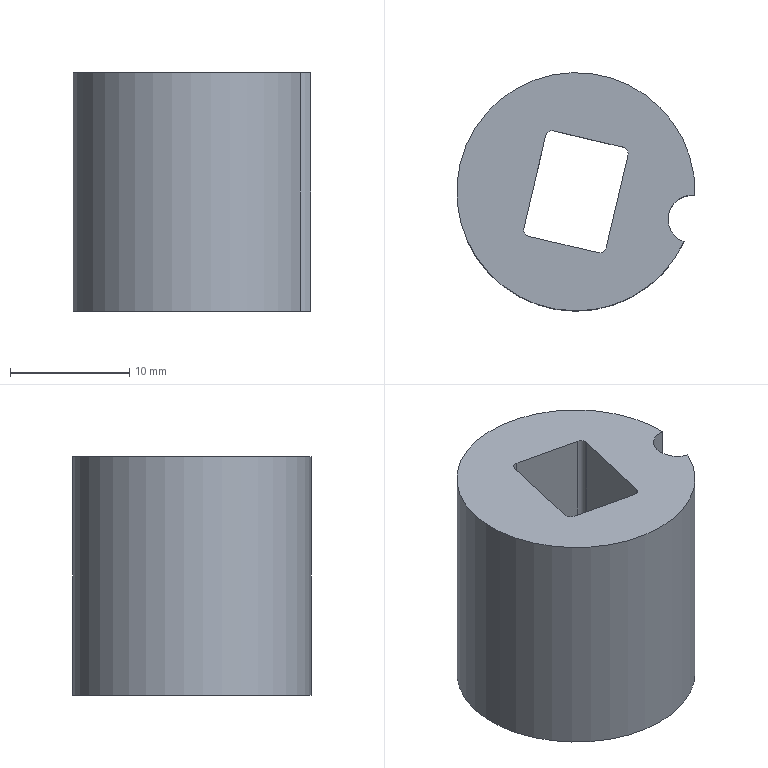Part | NX | features solid 2 | 1 solid | 14 faces | box 20 x 20 x 20 mm | volume 4152 mm3 | cylinder 7 | plane 7 | commonest cylinder face diameters 1.1 x4 4 x1 12.6 x1 20 x1
STEP:
#1=CARTESIAN_POINT('',(-482.896,-233.019,31.));
#2=VERTEX_POINT('',#1);
#3=CARTESIAN_POINT('',(-482.896,-233.019,51.));
#4=VERTEX_POINT('',#3);
#5=CARTESIAN_POINT('',(-482.896,-233.019,41.));
#6=DIRECTION('',(0.,0.,1.));
#7=VECTOR('',#6,1000.);
#8=LINE('',#5,#7);
#9=EDGE_CURVE('',#2,#4,#8,.T.);
#10=ORIENTED_EDGE('',*,*,#9,.F.);
#11=CARTESIAN_POINT('',(-483.808,-236.893,31.));
#12=VERTEX_POINT('',#11);
#13=CARTESIAN_POINT('',(-492.891,-232.711,31.));
#14=DIRECTION('',(0.,0.,1.));
#15=DIRECTION('',(0.9734,-0.2291,0.));
#16=AXIS2_PLACEMENT_3D('',#13,#14,#15);
#17=CIRCLE('',#16,10.);
#18=EDGE_CURVE('',#2,#12,#17,.T.);
#19=ORIENTED_EDGE('',*,*,#18,.T.);
#20=CARTESIAN_POINT('',(-483.808,-236.893,51.));
#21=VERTEX_POINT('',#20);
#22=CARTESIAN_POINT('',(-483.808,-236.893,41.));
#23=DIRECTION('',(0.,0.,1.));
#24=VECTOR('',#23,1000.);
#25=LINE('',#22,#24);
#26=EDGE_CURVE('',#21,#12,#25,.F.);
#27=ORIENTED_EDGE('',*,*,#26,.F.);
#28=CARTESIAN_POINT('',(-492.891,-232.711,51.));
#29=DIRECTION('',(0.,0.,1.));
#30=DIRECTION('',(0.9734,-0.2291,0.));
#31=AXIS2_PLACEMENT_3D('',#28,#29,#30);
#32=CIRCLE('',#31,10.);
#33=EDGE_CURVE('',#4,#21,#32,.T.);
#34=ORIENTED_EDGE('',*,*,#33,.F.);
#35=EDGE_LOOP('',(#10,#19,#27,#34));
#36=FACE_BOUND('',#35,.T.);
#37=CARTESIAN_POINT('',(-492.891,-232.711,31.));
#38=DIRECTION('',(0.,0.,1.));
#39=DIRECTION('',(0.9734,-0.2291,0.));
#40=AXIS2_PLACEMENT_3D('',#37,#38,#39);
#41=CYLINDRICAL_SURFACE('',#40,10.);
#42=ADVANCED_FACE('',(#36),#41,.T.);
#43=CARTESIAN_POINT('',(-486.759,-234.155,31.));
#44=VERTEX_POINT('',#43);
#45=CARTESIAN_POINT('',(-492.891,-232.711,31.));
#46=DIRECTION('',(0.,0.,1.));
#47=DIRECTION('',(0.9734,-0.2291,0.));
#48=AXIS2_PLACEMENT_3D('',#45,#46,#47);
#49=CIRCLE('',#48,6.3);
#50=EDGE_CURVE('',#44,#44,#49,.T.);
#51=ORIENTED_EDGE('',*,*,#50,.T.);
#52=EDGE_LOOP('',(#51));
#53=FACE_BOUND('',#52,.T.);
#54=ORIENTED_EDGE('',*,*,#18,.F.);
#55=CARTESIAN_POINT('',(-483.157,-235.002,31.));
#56=DIRECTION('',(0.,0.,1.));
#57=DIRECTION('',(0.9734,-0.2291,0.));
#58=AXIS2_PLACEMENT_3D('',#55,#56,#57);
#59=CIRCLE('',#58,2.);
#60=EDGE_CURVE('',#2,#12,#59,.T.);
#61=ORIENTED_EDGE('',*,*,#60,.T.);
#62=EDGE_LOOP('',(#54,#61));
#63=FACE_BOUND('',#62,.T.);
#64=CARTESIAN_POINT('',(-492.891,-232.711,31.));
#65=DIRECTION('',(0.,0.,1.));
#66=DIRECTION('',(0.9734,-0.2291,0.));
#67=AXIS2_PLACEMENT_3D('',#64,#65,#66);
#68=PLANE('',#67);
#69=ADVANCED_FACE('',(#53,#63),#68,.F.);
#70=CARTESIAN_POINT('',(-495.43,-228.004,51.));
#71=VERTEX_POINT('',#70);
#72=CARTESIAN_POINT('',(-497.263,-235.791,51.));
#73=VERTEX_POINT('',#72);
#74=CARTESIAN_POINT('',(-495.304,-227.469,51.));
#75=DIRECTION('',(-0.2291,-0.9734,0.));
#76=VECTOR('',#75,1000.);
#77=LINE('',#74,#76);
#78=EDGE_CURVE('',#71,#73,#77,.T.);
#79=ORIENTED_EDGE('',*,*,#78,.F.);
#80=CARTESIAN_POINT('',(-494.769,-227.595,51.));
#81=VERTEX_POINT('',#80);
#82=CARTESIAN_POINT('',(-494.895,-228.13,51.));
#83=DIRECTION('',(0.,0.,1.));
#84=DIRECTION('',(0.9734,-0.2291,0.));
#85=AXIS2_PLACEMENT_3D('',#82,#83,#84);
#86=CIRCLE('',#85,0.55);
#87=EDGE_CURVE('',#71,#81,#86,.F.);
#88=ORIENTED_EDGE('',*,*,#87,.T.);
#89=CARTESIAN_POINT('',(-488.929,-228.97,51.));
#90=VERTEX_POINT('',#89);
#91=CARTESIAN_POINT('',(-488.393,-229.096,51.));
#92=DIRECTION('',(-0.9734,0.2291,0.));
#93=VECTOR('',#92,1000.);
#94=LINE('',#91,#93);
#95=EDGE_CURVE('',#90,#81,#94,.T.);
#96=ORIENTED_EDGE('',*,*,#95,.F.);
#97=CARTESIAN_POINT('',(-488.519,-229.631,51.));
#98=VERTEX_POINT('',#97);
#99=CARTESIAN_POINT('',(-489.055,-229.505,51.));
#100=DIRECTION('',(0.,0.,1.));
#101=DIRECTION('',(0.9734,-0.2291,0.));
#102=AXIS2_PLACEMENT_3D('',#99,#100,#101);
#103=CIRCLE('',#102,0.55);
#104=EDGE_CURVE('',#90,#98,#103,.F.);
#105=ORIENTED_EDGE('',*,*,#104,.T.);
#106=CARTESIAN_POINT('',(-490.352,-237.418,51.));
#107=VERTEX_POINT('',#106);
#108=CARTESIAN_POINT('',(-488.393,-229.096,51.));
#109=DIRECTION('',(-0.2291,-0.9734,0.));
#110=VECTOR('',#109,1000.);
#111=LINE('',#108,#110);
#112=EDGE_CURVE('',#98,#107,#111,.T.);
#113=ORIENTED_EDGE('',*,*,#112,.T.);
#114=CARTESIAN_POINT('',(-491.014,-237.827,51.));
#115=VERTEX_POINT('',#114);
#116=CARTESIAN_POINT('',(-490.888,-237.292,51.));
#117=DIRECTION('',(0.,0.,1.));
#118=DIRECTION('',(0.9734,-0.2291,0.));
#119=AXIS2_PLACEMENT_3D('',#116,#117,#118);
#120=CIRCLE('',#119,0.55);
#121=EDGE_CURVE('',#107,#115,#120,.F.);
#122=ORIENTED_EDGE('',*,*,#121,.T.);
#123=CARTESIAN_POINT('',(-496.854,-236.453,51.));
#124=VERTEX_POINT('',#123);
#125=CARTESIAN_POINT('',(-497.389,-236.327,51.));
#126=DIRECTION('',(0.9734,-0.2291,0.));
#127=VECTOR('',#126,1000.);
#128=LINE('',#125,#127);
#129=EDGE_CURVE('',#124,#115,#128,.T.);
#130=ORIENTED_EDGE('',*,*,#129,.F.);
#131=CARTESIAN_POINT('',(-496.728,-235.917,51.));
#132=DIRECTION('',(0.,0.,1.));
#133=DIRECTION('',(0.9734,-0.2291,0.));
#134=AXIS2_PLACEMENT_3D('',#131,#132,#133);
#135=CIRCLE('',#134,0.55);
#136=EDGE_CURVE('',#124,#73,#135,.F.);
#137=ORIENTED_EDGE('',*,*,#136,.T.);
#138=EDGE_LOOP('',(#79,#88,#96,#105,#113,#122,#130,#137));
#139=FACE_BOUND('',#138,.T.);
#140=CARTESIAN_POINT('',(-483.157,-235.002,51.));
#141=DIRECTION('',(0.,0.,1.));
#142=DIRECTION('',(0.9734,-0.2291,0.));
#143=AXIS2_PLACEMENT_3D('',#140,#141,#142);
#144=CIRCLE('',#143,2.);
#145=EDGE_CURVE('',#4,#21,#144,.T.);
#146=ORIENTED_EDGE('',*,*,#145,.F.);
#147=ORIENTED_EDGE('',*,*,#33,.T.);
#148=EDGE_LOOP('',(#146,#147));
#149=FACE_BOUND('',#148,.T.);
#150=CARTESIAN_POINT('',(-492.891,-232.711,51.));
#151=DIRECTION('',(0.,0.,1.));
#152=DIRECTION('',(0.9734,-0.2291,0.));
#153=AXIS2_PLACEMENT_3D('',#150,#151,#152);
#154=PLANE('',#153);
#155=ADVANCED_FACE('',(#139,#149),#154,.T.);
#156=ORIENTED_EDGE('',*,*,#50,.F.);
#157=EDGE_LOOP('',(#156));
#158=FACE_BOUND('',#157,.T.);
#159=CARTESIAN_POINT('',(-486.759,-234.155,43.));
#160=VERTEX_POINT('',#159);
#161=CARTESIAN_POINT('',(-492.891,-232.711,43.));
#162=DIRECTION('',(0.,0.,1.));
#163=DIRECTION('',(0.9734,-0.2291,0.));
#164=AXIS2_PLACEMENT_3D('',#161,#162,#163);
#165=CIRCLE('',#164,6.3);
#166=EDGE_CURVE('',#160,#160,#165,.T.);
#167=ORIENTED_EDGE('',*,*,#166,.T.);
#168=EDGE_LOOP('',(#167));
#169=FACE_BOUND('',#168,.T.);
#170=CARTESIAN_POINT('',(-492.891,-232.711,31.));
#171=DIRECTION('',(0.,0.,1.));
#172=DIRECTION('',(0.9734,-0.2291,0.));
#173=AXIS2_PLACEMENT_3D('',#170,#171,#172);
#174=CYLINDRICAL_SURFACE('',#173,6.3);
#175=ADVANCED_FACE('',(#158,#169),#174,.F.);
#176=CARTESIAN_POINT('',(-488.519,-229.631,43.));
#177=VERTEX_POINT('',#176);
#178=CARTESIAN_POINT('',(-490.352,-237.418,43.));
#179=VERTEX_POINT('',#178);
#180=CARTESIAN_POINT('',(-489.436,-233.524,43.));
#181=DIRECTION('',(-0.2291,-0.9734,0.));
#182=VECTOR('',#181,1000.);
#183=LINE('',#180,#182);
#184=EDGE_CURVE('',#177,#179,#183,.T.);
#185=ORIENTED_EDGE('',*,*,#184,.F.);
#186=CARTESIAN_POINT('',(-488.929,-228.97,43.));
#187=VERTEX_POINT('',#186);
#188=CARTESIAN_POINT('',(-489.055,-229.505,43.));
#189=DIRECTION('',(0.,0.,1.));
#190=DIRECTION('',(0.9734,-0.2291,0.));
#191=AXIS2_PLACEMENT_3D('',#188,#189,#190);
#192=CIRCLE('',#191,0.55);
#193=EDGE_CURVE('',#177,#187,#192,.T.);
#194=ORIENTED_EDGE('',*,*,#193,.T.);
#195=CARTESIAN_POINT('',(-494.769,-227.595,43.));
#196=VERTEX_POINT('',#195);
#197=CARTESIAN_POINT('',(-491.849,-228.282,43.));
#198=DIRECTION('',(-0.9734,0.2291,0.));
#199=VECTOR('',#198,1000.);
#200=LINE('',#197,#199);
#201=EDGE_CURVE('',#187,#196,#200,.T.);
#202=ORIENTED_EDGE('',*,*,#201,.T.);
#203=CARTESIAN_POINT('',(-495.43,-228.004,43.));
#204=VERTEX_POINT('',#203);
#205=CARTESIAN_POINT('',(-494.895,-228.13,43.));
#206=DIRECTION('',(0.,0.,1.));
#207=DIRECTION('',(0.9734,-0.2291,0.));
#208=AXIS2_PLACEMENT_3D('',#205,#206,#207);
#209=CIRCLE('',#208,0.55);
#210=EDGE_CURVE('',#196,#204,#209,.T.);
#211=ORIENTED_EDGE('',*,*,#210,.T.);
#212=CARTESIAN_POINT('',(-497.263,-235.791,43.));
#213=VERTEX_POINT('',#212);
#214=CARTESIAN_POINT('',(-496.347,-231.898,43.));
#215=DIRECTION('',(-0.2291,-0.9734,0.));
#216=VECTOR('',#215,1000.);
#217=LINE('',#214,#216);
#218=EDGE_CURVE('',#204,#213,#217,.T.);
#219=ORIENTED_EDGE('',*,*,#218,.T.);
#220=CARTESIAN_POINT('',(-496.854,-236.453,43.));
#221=VERTEX_POINT('',#220);
#222=CARTESIAN_POINT('',(-496.728,-235.917,43.));
#223=DIRECTION('',(0.,0.,1.));
#224=DIRECTION('',(0.9734,-0.2291,0.));
#225=AXIS2_PLACEMENT_3D('',#222,#223,#224);
#226=CIRCLE('',#225,0.55);
#227=EDGE_CURVE('',#213,#221,#226,.T.);
#228=ORIENTED_EDGE('',*,*,#227,.T.);
#229=CARTESIAN_POINT('',(-491.014,-237.827,43.));
#230=VERTEX_POINT('',#229);
#231=CARTESIAN_POINT('',(-493.934,-237.14,43.));
#232=DIRECTION('',(0.9734,-0.2291,0.));
#233=VECTOR('',#232,1000.);
#234=LINE('',#231,#233);
#235=EDGE_CURVE('',#221,#230,#234,.T.);
#236=ORIENTED_EDGE('',*,*,#235,.T.);
#237=CARTESIAN_POINT('',(-490.888,-237.292,43.));
#238=DIRECTION('',(0.,0.,1.));
#239=DIRECTION('',(0.9734,-0.2291,0.));
#240=AXIS2_PLACEMENT_3D('',#237,#238,#239);
#241=CIRCLE('',#240,0.55);
#242=EDGE_CURVE('',#230,#179,#241,.T.);
#243=ORIENTED_EDGE('',*,*,#242,.T.);
#244=EDGE_LOOP('',(#185,#194,#202,#211,#219,#228,#236,#243));
#245=FACE_BOUND('',#244,.T.);
#246=ORIENTED_EDGE('',*,*,#166,.F.);
#247=EDGE_LOOP('',(#246));
#248=FACE_BOUND('',#247,.T.);
#249=CARTESIAN_POINT('',(-492.891,-232.711,43.));
#250=DIRECTION('',(0.,0.,1.));
#251=DIRECTION('',(0.9734,-0.2291,0.));
#252=AXIS2_PLACEMENT_3D('',#249,#250,#251);
#253=PLANE('',#252);
#254=ADVANCED_FACE('',(#245,#248),#253,.F.);
#255=ORIENTED_EDGE('',*,*,#9,.T.);
#256=ORIENTED_EDGE('',*,*,#145,.T.);
#257=ORIENTED_EDGE('',*,*,#26,.T.);
#258=ORIENTED_EDGE('',*,*,#60,.F.);
#259=EDGE_LOOP('',(#255,#256,#257,#258));
#260=FACE_BOUND('',#259,.T.);
#261=CARTESIAN_POINT('',(-483.157,-235.002,31.));
#262=DIRECTION('',(0.,0.,1.));
#263=DIRECTION('',(0.9734,-0.2291,0.));
#264=AXIS2_PLACEMENT_3D('',#261,#262,#263);
#265=CYLINDRICAL_SURFACE('',#264,2.);
#266=ADVANCED_FACE('',(#260),#265,.F.);
#267=ORIENTED_EDGE('',*,*,#78,.T.);
#268=CARTESIAN_POINT('',(-497.263,-235.791,43.));
#269=DIRECTION('',(0.,0.,1.));
#270=VECTOR('',#269,1000.);
#271=LINE('',#268,#270);
#272=EDGE_CURVE('',#73,#213,#271,.F.);
#273=ORIENTED_EDGE('',*,*,#272,.T.);
#274=ORIENTED_EDGE('',*,*,#218,.F.);
#275=CARTESIAN_POINT('',(-495.43,-228.004,51.));
#276=DIRECTION('',(0.,0.,1.));
#277=VECTOR('',#276,1000.);
#278=LINE('',#275,#277);
#279=EDGE_CURVE('',#204,#71,#278,.T.);
#280=ORIENTED_EDGE('',*,*,#279,.T.);
#281=EDGE_LOOP('',(#267,#273,#274,#280));
#282=FACE_BOUND('',#281,.T.);
#283=CARTESIAN_POINT('',(-495.304,-227.469,31.));
#284=DIRECTION('',(-0.9734,0.2291,0.));
#285=DIRECTION('',(0.,0.,1.));
#286=AXIS2_PLACEMENT_3D('',#283,#284,#285);
#287=PLANE('',#286);
#288=ADVANCED_FACE('',(#282),#287,.F.);
#289=ORIENTED_EDGE('',*,*,#129,.T.);
#290=CARTESIAN_POINT('',(-491.014,-237.827,31.));
#291=DIRECTION('',(0.,0.,1.));
#292=VECTOR('',#291,1000.);
#293=LINE('',#290,#292);
#294=EDGE_CURVE('',#115,#230,#293,.F.);
#295=ORIENTED_EDGE('',*,*,#294,.T.);
#296=ORIENTED_EDGE('',*,*,#235,.F.);
#297=CARTESIAN_POINT('',(-496.854,-236.453,51.));
#298=DIRECTION('',(0.,0.,1.));
#299=VECTOR('',#298,1000.);
#300=LINE('',#297,#299);
#301=EDGE_CURVE('',#221,#124,#300,.T.);
#302=ORIENTED_EDGE('',*,*,#301,.T.);
#303=EDGE_LOOP('',(#289,#295,#296,#302));
#304=FACE_BOUND('',#303,.T.);
#305=CARTESIAN_POINT('',(-497.389,-236.327,31.));
#306=DIRECTION('',(-0.2291,-0.9734,0.));
#307=DIRECTION('',(0.,0.,-1.));
#308=AXIS2_PLACEMENT_3D('',#305,#306,#307);
#309=PLANE('',#308);
#310=ADVANCED_FACE('',(#304),#309,.F.);
#311=ORIENTED_EDGE('',*,*,#112,.F.);
#312=CARTESIAN_POINT('',(-488.519,-229.631,31.));
#313=DIRECTION('',(0.,0.,1.));
#314=VECTOR('',#313,1000.);
#315=LINE('',#312,#314);
#316=EDGE_CURVE('',#98,#177,#315,.F.);
#317=ORIENTED_EDGE('',*,*,#316,.T.);
#318=ORIENTED_EDGE('',*,*,#184,.T.);
#319=CARTESIAN_POINT('',(-490.352,-237.418,31.));
#320=DIRECTION('',(0.,0.,1.));
#321=VECTOR('',#320,1000.);
#322=LINE('',#319,#321);
#323=EDGE_CURVE('',#179,#107,#322,.T.);
#324=ORIENTED_EDGE('',*,*,#323,.T.);
#325=EDGE_LOOP('',(#311,#317,#318,#324));
#326=FACE_BOUND('',#325,.T.);
#327=CARTESIAN_POINT('',(-488.393,-229.096,31.));
#328=DIRECTION('',(-0.9734,0.2291,0.));
#329=DIRECTION('',(0.,0.,1.));
#330=AXIS2_PLACEMENT_3D('',#327,#328,#329);
#331=PLANE('',#330);
#332=ADVANCED_FACE('',(#326),#331,.T.);
#333=ORIENTED_EDGE('',*,*,#201,.F.);
#334=CARTESIAN_POINT('',(-488.929,-228.97,31.));
#335=DIRECTION('',(0.,0.,1.));
#336=VECTOR('',#335,1000.);
#337=LINE('',#334,#336);
#338=EDGE_CURVE('',#187,#90,#337,.T.);
#339=ORIENTED_EDGE('',*,*,#338,.T.);
#340=ORIENTED_EDGE('',*,*,#95,.T.);
#341=CARTESIAN_POINT('',(-494.769,-227.595,43.));
#342=DIRECTION('',(0.,0.,1.));
#343=VECTOR('',#342,1000.);
#344=LINE('',#341,#343);
#345=EDGE_CURVE('',#81,#196,#344,.F.);
#346=ORIENTED_EDGE('',*,*,#345,.T.);
#347=EDGE_LOOP('',(#333,#339,#340,#346));
#348=FACE_BOUND('',#347,.T.);
#349=CARTESIAN_POINT('',(-488.393,-229.096,31.));
#350=DIRECTION('',(0.2291,0.9734,0.));
#351=DIRECTION('',(0.,0.,1.));
#352=AXIS2_PLACEMENT_3D('',#349,#350,#351);
#353=PLANE('',#352);
#354=ADVANCED_FACE('',(#348),#353,.F.);
#355=ORIENTED_EDGE('',*,*,#193,.F.);
#356=ORIENTED_EDGE('',*,*,#316,.F.);
#357=ORIENTED_EDGE('',*,*,#104,.F.);
#358=ORIENTED_EDGE('',*,*,#338,.F.);
#359=EDGE_LOOP('',(#355,#356,#357,#358));
#360=FACE_BOUND('',#359,.T.);
#361=CARTESIAN_POINT('',(-489.055,-229.505,31.));
#362=DIRECTION('',(0.,0.,1.));
#363=DIRECTION('',(0.9734,-0.2291,0.));
#364=AXIS2_PLACEMENT_3D('',#361,#362,#363);
#365=CYLINDRICAL_SURFACE('',#364,0.55);
#366=ADVANCED_FACE('',(#360),#365,.F.);
#367=ORIENTED_EDGE('',*,*,#242,.F.);
#368=ORIENTED_EDGE('',*,*,#294,.F.);
#369=ORIENTED_EDGE('',*,*,#121,.F.);
#370=ORIENTED_EDGE('',*,*,#323,.F.);
#371=EDGE_LOOP('',(#367,#368,#369,#370));
#372=FACE_BOUND('',#371,.T.);
#373=CARTESIAN_POINT('',(-490.888,-237.292,31.));
#374=DIRECTION('',(0.,0.,1.));
#375=DIRECTION('',(0.9734,-0.2291,0.));
#376=AXIS2_PLACEMENT_3D('',#373,#374,#375);
#377=CYLINDRICAL_SURFACE('',#376,0.55);
#378=ADVANCED_FACE('',(#372),#377,.F.);
#379=ORIENTED_EDGE('',*,*,#227,.F.);
#380=ORIENTED_EDGE('',*,*,#272,.F.);
#381=ORIENTED_EDGE('',*,*,#136,.F.);
#382=ORIENTED_EDGE('',*,*,#301,.F.);
#383=EDGE_LOOP('',(#379,#380,#381,#382));
#384=FACE_BOUND('',#383,.T.);
#385=CARTESIAN_POINT('',(-496.728,-235.917,31.));
#386=DIRECTION('',(0.,0.,-1.));
#387=DIRECTION('',(-0.9734,0.2291,0.));
#388=AXIS2_PLACEMENT_3D('',#385,#386,#387);
#389=CYLINDRICAL_SURFACE('',#388,0.55);
#390=ADVANCED_FACE('',(#384),#389,.F.);
#391=ORIENTED_EDGE('',*,*,#210,.F.);
#392=ORIENTED_EDGE('',*,*,#345,.F.);
#393=ORIENTED_EDGE('',*,*,#87,.F.);
#394=ORIENTED_EDGE('',*,*,#279,.F.);
#395=EDGE_LOOP('',(#391,#392,#393,#394));
#396=FACE_BOUND('',#395,.T.);
#397=CARTESIAN_POINT('',(-494.895,-228.13,31.));
#398=DIRECTION('',(0.,0.,-1.));
#399=DIRECTION('',(-0.9734,0.2291,0.));
#400=AXIS2_PLACEMENT_3D('',#397,#398,#399);
#401=CYLINDRICAL_SURFACE('',#400,0.55);
#402=ADVANCED_FACE('',(#396),#401,.F.);
#403=CLOSED_SHELL('',(#42,#69,#155,#175,#254,#266,#288,#310,#332,#354,#366,#378,#390,#402));
#404=MANIFOLD_SOLID_BREP('',#403);
#405=(LENGTH_UNIT()NAMED_UNIT(*)SI_UNIT(.MILLI.,.METRE.));
#406=UNCERTAINTY_MEASURE_WITH_UNIT(LENGTH_MEASURE(0.00001),#405,'','');
#407=(NAMED_UNIT(*)PLANE_ANGLE_UNIT()SI_UNIT($,.RADIAN.));
#408=(NAMED_UNIT(*)SI_UNIT($,.STERADIAN.)SOLID_ANGLE_UNIT());
#409=(GEOMETRIC_REPRESENTATION_CONTEXT(3)GLOBAL_UNCERTAINTY_ASSIGNED_CONTEXT((#406))GLOBAL_UNIT_ASSIGNED_CONTEXT((#405,#407,#408))REPRESENTATION_CONTEXT('',''));
#410=ADVANCED_BREP_SHAPE_REPRESENTATION('',(#404),#409);